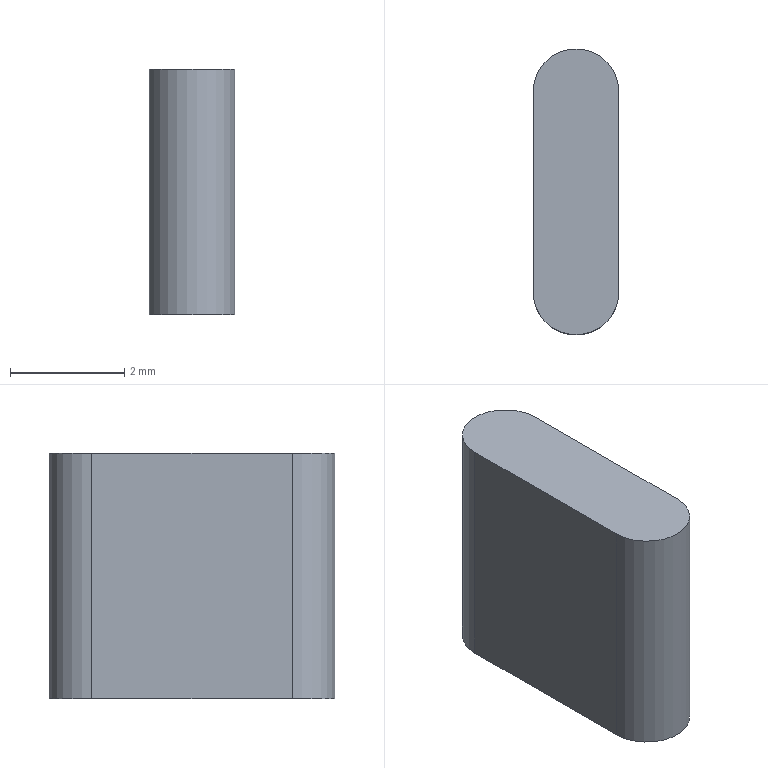Part | SolidWorks | features Extrusion 1 | 1 solid | 6 faces | box 1.5 x 5 x 4.3 mm | volume 30.174 mm3 | plane 4 | cylinder 2 | commonest cylinder face diameters 1.5 x2
STEP:
#1=CARTESIAN_POINT('',(-0.75,-1.75,-2.15));
#2=VERTEX_POINT('',#1);
#3=CARTESIAN_POINT('',(0.75,-1.75,-2.15));
#4=VERTEX_POINT('',#3);
#5=CARTESIAN_POINT('',(0.,-1.75,-2.15));
#6=DIRECTION('',(0.,0.,1.));
#7=DIRECTION('',(1.,0.,0.));
#8=AXIS2_PLACEMENT_3D('',#5,#6,#7);
#9=CIRCLE('',#8,0.75);
#10=EDGE_CURVE('',#2,#4,#9,.T.);
#11=ORIENTED_EDGE('',*,*,#10,.T.);
#12=CARTESIAN_POINT('',(0.75,-1.75,2.15));
#13=VERTEX_POINT('',#12);
#14=CARTESIAN_POINT('',(0.75,-1.75,2.15));
#15=DIRECTION('',(0.,0.,-1.));
#16=VECTOR('',#15,1000.);
#17=LINE('',#14,#16);
#18=EDGE_CURVE('',#13,#4,#17,.T.);
#19=ORIENTED_EDGE('',*,*,#18,.F.);
#20=CARTESIAN_POINT('',(-0.75,-1.75,2.15));
#21=VERTEX_POINT('',#20);
#22=CARTESIAN_POINT('',(0.,-1.75,2.15));
#23=DIRECTION('',(0.,0.,1.));
#24=DIRECTION('',(1.,0.,0.));
#25=AXIS2_PLACEMENT_3D('',#22,#23,#24);
#26=CIRCLE('',#25,0.75);
#27=EDGE_CURVE('',#21,#13,#26,.T.);
#28=ORIENTED_EDGE('',*,*,#27,.F.);
#29=CARTESIAN_POINT('',(-0.75,-1.75,2.15));
#30=DIRECTION('',(0.,0.,-1.));
#31=VECTOR('',#30,1000.);
#32=LINE('',#29,#31);
#33=EDGE_CURVE('',#21,#2,#32,.T.);
#34=ORIENTED_EDGE('',*,*,#33,.T.);
#35=EDGE_LOOP('',(#11,#19,#28,#34));
#36=FACE_OUTER_BOUND('',#35,.T.);
#37=CARTESIAN_POINT('',(0.,-1.75,2.15));
#38=DIRECTION('',(0.,0.,-1.));
#39=DIRECTION('',(-1.,0.,0.));
#40=AXIS2_PLACEMENT_3D('',#37,#38,#39);
#41=CYLINDRICAL_SURFACE('',#40,0.75);
#42=ADVANCED_FACE('',(#36),#41,.T.);
#43=CARTESIAN_POINT('',(0.75,1.75,-2.15));
#44=VERTEX_POINT('',#43);
#45=CARTESIAN_POINT('',(0.75,-1.75,-2.15));
#46=DIRECTION('',(0.,1.,0.));
#47=VECTOR('',#46,1000.);
#48=LINE('',#45,#47);
#49=EDGE_CURVE('',#4,#44,#48,.T.);
#50=ORIENTED_EDGE('',*,*,#49,.T.);
#51=CARTESIAN_POINT('',(0.75,1.75,2.15));
#52=VERTEX_POINT('',#51);
#53=CARTESIAN_POINT('',(0.75,1.75,2.15));
#54=DIRECTION('',(0.,0.,-1.));
#55=VECTOR('',#54,1000.);
#56=LINE('',#53,#55);
#57=EDGE_CURVE('',#52,#44,#56,.T.);
#58=ORIENTED_EDGE('',*,*,#57,.F.);
#59=CARTESIAN_POINT('',(0.75,-1.75,2.15));
#60=DIRECTION('',(0.,1.,0.));
#61=VECTOR('',#60,1000.);
#62=LINE('',#59,#61);
#63=EDGE_CURVE('',#13,#52,#62,.T.);
#64=ORIENTED_EDGE('',*,*,#63,.F.);
#65=ORIENTED_EDGE('',*,*,#18,.T.);
#66=EDGE_LOOP('',(#50,#58,#64,#65));
#67=FACE_OUTER_BOUND('',#66,.T.);
#68=CARTESIAN_POINT('',(0.75,-1.75,2.15));
#69=DIRECTION('',(-1.,0.,0.));
#70=DIRECTION('',(0.,-1.,0.));
#71=AXIS2_PLACEMENT_3D('',#68,#69,#70);
#72=PLANE('',#71);
#73=ADVANCED_FACE('',(#67),#72,.F.);
#74=CARTESIAN_POINT('',(-0.75,1.75,-2.15));
#75=VERTEX_POINT('',#74);
#76=CARTESIAN_POINT('',(0.,1.75,-2.15));
#77=DIRECTION('',(0.,0.,1.));
#78=DIRECTION('',(1.,0.,0.));
#79=AXIS2_PLACEMENT_3D('',#76,#77,#78);
#80=CIRCLE('',#79,0.75);
#81=EDGE_CURVE('',#44,#75,#80,.T.);
#82=ORIENTED_EDGE('',*,*,#81,.T.);
#83=CARTESIAN_POINT('',(-0.75,1.75,2.15));
#84=VERTEX_POINT('',#83);
#85=CARTESIAN_POINT('',(-0.75,1.75,2.15));
#86=DIRECTION('',(0.,0.,-1.));
#87=VECTOR('',#86,1000.);
#88=LINE('',#85,#87);
#89=EDGE_CURVE('',#84,#75,#88,.T.);
#90=ORIENTED_EDGE('',*,*,#89,.F.);
#91=CARTESIAN_POINT('',(0.,1.75,2.15));
#92=DIRECTION('',(0.,0.,1.));
#93=DIRECTION('',(1.,0.,0.));
#94=AXIS2_PLACEMENT_3D('',#91,#92,#93);
#95=CIRCLE('',#94,0.75);
#96=EDGE_CURVE('',#52,#84,#95,.T.);
#97=ORIENTED_EDGE('',*,*,#96,.F.);
#98=ORIENTED_EDGE('',*,*,#57,.T.);
#99=EDGE_LOOP('',(#82,#90,#97,#98));
#100=FACE_OUTER_BOUND('',#99,.T.);
#101=CARTESIAN_POINT('',(0.,1.75,2.15));
#102=DIRECTION('',(0.,0.,-1.));
#103=DIRECTION('',(-1.,0.,0.));
#104=AXIS2_PLACEMENT_3D('',#101,#102,#103);
#105=CYLINDRICAL_SURFACE('',#104,0.75);
#106=ADVANCED_FACE('',(#100),#105,.T.);
#107=CARTESIAN_POINT('',(-0.75,-1.75,-2.15));
#108=DIRECTION('',(0.,-1.,0.));
#109=VECTOR('',#108,1000.);
#110=LINE('',#107,#109);
#111=EDGE_CURVE('',#75,#2,#110,.T.);
#112=ORIENTED_EDGE('',*,*,#111,.T.);
#113=ORIENTED_EDGE('',*,*,#33,.F.);
#114=CARTESIAN_POINT('',(-0.75,-1.75,2.15));
#115=DIRECTION('',(0.,-1.,0.));
#116=VECTOR('',#115,1000.);
#117=LINE('',#114,#116);
#118=EDGE_CURVE('',#84,#21,#117,.T.);
#119=ORIENTED_EDGE('',*,*,#118,.F.);
#120=ORIENTED_EDGE('',*,*,#89,.T.);
#121=EDGE_LOOP('',(#112,#113,#119,#120));
#122=FACE_OUTER_BOUND('',#121,.T.);
#123=CARTESIAN_POINT('',(-0.75,-1.75,2.15));
#124=DIRECTION('',(1.,0.,0.));
#125=DIRECTION('',(0.,1.,0.));
#126=AXIS2_PLACEMENT_3D('',#123,#124,#125);
#127=PLANE('',#126);
#128=ADVANCED_FACE('',(#122),#127,.F.);
#129=ORIENTED_EDGE('',*,*,#27,.T.);
#130=ORIENTED_EDGE('',*,*,#63,.T.);
#131=ORIENTED_EDGE('',*,*,#96,.T.);
#132=ORIENTED_EDGE('',*,*,#118,.T.);
#133=EDGE_LOOP('',(#129,#130,#131,#132));
#134=FACE_OUTER_BOUND('',#133,.T.);
#135=CARTESIAN_POINT('',(0.,-1.75,2.15));
#136=DIRECTION('',(0.,0.,1.));
#137=DIRECTION('',(1.,0.,0.));
#138=AXIS2_PLACEMENT_3D('',#135,#136,#137);
#139=PLANE('',#138);
#140=ADVANCED_FACE('',(#134),#139,.T.);
#141=ORIENTED_EDGE('',*,*,#10,.F.);
#142=ORIENTED_EDGE('',*,*,#111,.F.);
#143=ORIENTED_EDGE('',*,*,#81,.F.);
#144=ORIENTED_EDGE('',*,*,#49,.F.);
#145=EDGE_LOOP('',(#141,#142,#143,#144));
#146=FACE_OUTER_BOUND('',#145,.T.);
#147=CARTESIAN_POINT('',(0.,-1.75,-2.15));
#148=DIRECTION('',(0.,0.,1.));
#149=DIRECTION('',(1.,0.,0.));
#150=AXIS2_PLACEMENT_3D('',#147,#148,#149);
#151=PLANE('',#150);
#152=ADVANCED_FACE('',(#146),#151,.F.);
#153=CLOSED_SHELL('',(#42,#73,#106,#128,#140,#152));
#154=MANIFOLD_SOLID_BREP('',#153);
#155=CARTESIAN_POINT('',(0.,0.,0.));
#156=DIRECTION('',(0.,0.,1.));
#157=DIRECTION('',(1.,0.,0.));
#158=AXIS2_PLACEMENT_3D('',#155,#156,#157);
#159=(LENGTH_UNIT()NAMED_UNIT(*)SI_UNIT(.MILLI.,.METRE.));
#160=UNCERTAINTY_MEASURE_WITH_UNIT(LENGTH_MEASURE(0.00001),#159,'','');
#161=(NAMED_UNIT(*)PLANE_ANGLE_UNIT()SI_UNIT($,.RADIAN.));
#162=(NAMED_UNIT(*)SI_UNIT($,.STERADIAN.)SOLID_ANGLE_UNIT());
#163=(GEOMETRIC_REPRESENTATION_CONTEXT(3)GLOBAL_UNCERTAINTY_ASSIGNED_CONTEXT((#160))GLOBAL_UNIT_ASSIGNED_CONTEXT((#159,#161,#162))REPRESENTATION_CONTEXT('',''));
#164=ADVANCED_BREP_SHAPE_REPRESENTATION('',(#154,#158),#163);